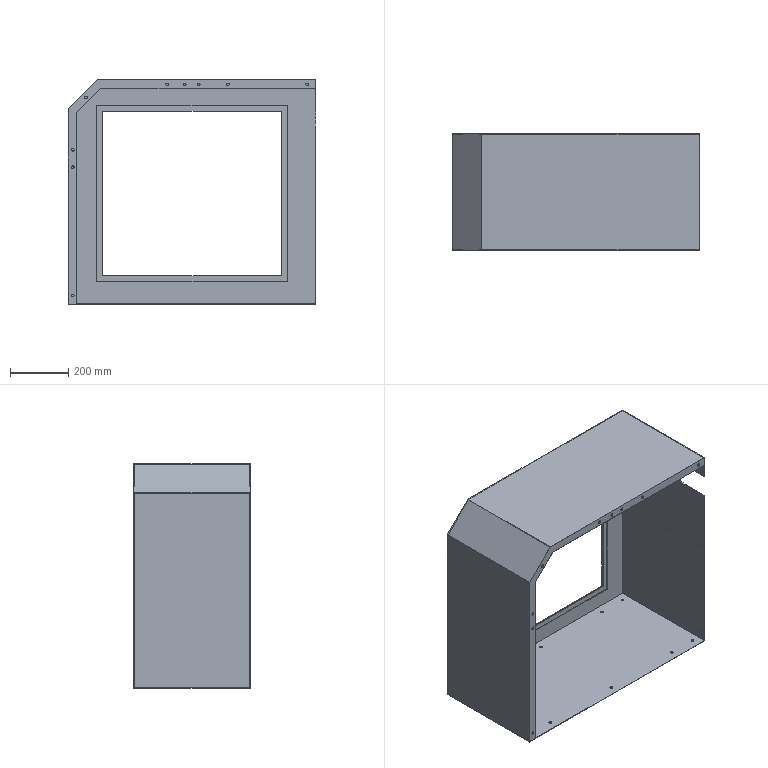Part | SolidWorks | features ICE 9, Extrusion 1, HoleWzd 1, Shell 1 | 1 solid | 90 faces | box 850 x 400 x 770 mm | volume 3305317 mm3 | cylinder 57 | plane 33 | commonest cylinder face diameters 9 x50 4.2 x6 80 x1